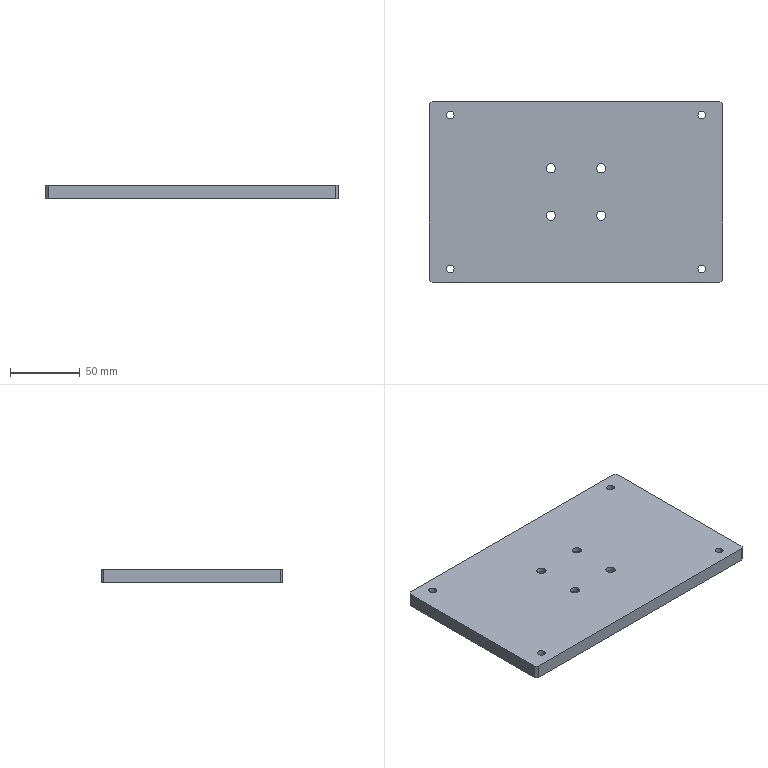Part | SolidWorks | features 3DProfileFeature 2, HoleWzd 2, Chamfer 1, Extrusion 1 | 1 solid | 50 faces | box 210 x 130 x 10 mm | volume 267698 mm3 | cylinder 32 | plane 18 | commonest cylinder face diameters 5.5 x8 6.6 x8 10 x8 11 x8
STEP:
#1=CARTESIAN_POINT('',(-85.,-55.,5.7));
#2=VERTEX_POINT('',#1);
#3=CARTESIAN_POINT('',(-95.,-55.,5.7));
#4=VERTEX_POINT('',#3);
#5=CARTESIAN_POINT('',(-90.,-55.,5.7));
#6=DIRECTION('',(0.,0.,-1.));
#7=DIRECTION('',(-1.,0.,0.));
#8=AXIS2_PLACEMENT_3D('',#5,#6,#7);
#9=CIRCLE('',#8,5.);
#10=EDGE_CURVE('',#2,#4,#9,.T.);
#11=ORIENTED_EDGE('',*,*,#10,.F.);
#12=CARTESIAN_POINT('',(-85.,-55.,0.));
#13=VERTEX_POINT('',#12);
#14=CARTESIAN_POINT('',(-85.,-55.,0.));
#15=DIRECTION('',(0.,0.,-1.));
#16=VECTOR('',#15,1000.);
#17=LINE('',#14,#16);
#18=EDGE_CURVE('',#2,#13,#17,.T.);
#19=ORIENTED_EDGE('',*,*,#18,.T.);
#20=CARTESIAN_POINT('',(-95.,-55.,0.));
#21=VERTEX_POINT('',#20);
#22=CARTESIAN_POINT('',(-90.,-55.,0.));
#23=DIRECTION('',(0.,0.,-1.));
#24=DIRECTION('',(-1.,0.,0.));
#25=AXIS2_PLACEMENT_3D('',#22,#23,#24);
#26=CIRCLE('',#25,5.);
#27=EDGE_CURVE('',#13,#21,#26,.T.);
#28=ORIENTED_EDGE('',*,*,#27,.T.);
#29=CARTESIAN_POINT('',(-95.,-55.,0.));
#30=DIRECTION('',(0.,0.,-1.));
#31=VECTOR('',#30,1000.);
#32=LINE('',#29,#31);
#33=EDGE_CURVE('',#4,#21,#32,.T.);
#34=ORIENTED_EDGE('',*,*,#33,.F.);
#35=EDGE_LOOP('',(#11,#19,#28,#34));
#36=FACE_OUTER_BOUND('',#35,.T.);
#37=CARTESIAN_POINT('',(-90.,-55.,0.));
#38=DIRECTION('',(0.,0.,-1.));
#39=DIRECTION('',(-1.,0.,0.));
#40=AXIS2_PLACEMENT_3D('',#37,#38,#39);
#41=CYLINDRICAL_SURFACE('',#40,5.);
#42=ADVANCED_FACE('',(#36),#41,.F.);
#43=CARTESIAN_POINT('',(-87.25,-55.,10.));
#44=VERTEX_POINT('',#43);
#45=CARTESIAN_POINT('',(-92.75,-55.,10.));
#46=VERTEX_POINT('',#45);
#47=CARTESIAN_POINT('',(-90.,-55.,10.));
#48=DIRECTION('',(0.,0.,-1.));
#49=DIRECTION('',(-1.,0.,0.));
#50=AXIS2_PLACEMENT_3D('',#47,#48,#49);
#51=CIRCLE('',#50,2.75);
#52=EDGE_CURVE('',#44,#46,#51,.T.);
#53=ORIENTED_EDGE('',*,*,#52,.F.);
#54=CARTESIAN_POINT('',(-87.25,-55.,5.7));
#55=VERTEX_POINT('',#54);
#56=CARTESIAN_POINT('',(-87.25,-55.,0.));
#57=DIRECTION('',(0.,0.,-1.));
#58=VECTOR('',#57,1000.);
#59=LINE('',#56,#58);
#60=EDGE_CURVE('',#44,#55,#59,.T.);
#61=ORIENTED_EDGE('',*,*,#60,.T.);
#62=CARTESIAN_POINT('',(-92.75,-55.,5.7));
#63=VERTEX_POINT('',#62);
#64=CARTESIAN_POINT('',(-90.,-55.,5.7));
#65=DIRECTION('',(0.,0.,-1.));
#66=DIRECTION('',(-1.,0.,0.));
#67=AXIS2_PLACEMENT_3D('',#64,#65,#66);
#68=CIRCLE('',#67,2.75);
#69=EDGE_CURVE('',#55,#63,#68,.T.);
#70=ORIENTED_EDGE('',*,*,#69,.T.);
#71=CARTESIAN_POINT('',(-92.75,-55.,0.));
#72=DIRECTION('',(0.,0.,-1.));
#73=VECTOR('',#72,1000.);
#74=LINE('',#71,#73);
#75=EDGE_CURVE('',#46,#63,#74,.T.);
#76=ORIENTED_EDGE('',*,*,#75,.F.);
#77=EDGE_LOOP('',(#53,#61,#70,#76));
#78=FACE_OUTER_BOUND('',#77,.T.);
#79=CARTESIAN_POINT('',(-90.,-55.,0.));
#80=DIRECTION('',(0.,0.,-1.));
#81=DIRECTION('',(-1.,0.,0.));
#82=AXIS2_PLACEMENT_3D('',#79,#80,#81);
#83=CYLINDRICAL_SURFACE('',#82,2.75);
#84=ADVANCED_FACE('',(#78),#83,.F.);
#85=CARTESIAN_POINT('',(-85.,55.,5.7));
#86=VERTEX_POINT('',#85);
#87=CARTESIAN_POINT('',(-95.,55.,5.7));
#88=VERTEX_POINT('',#87);
#89=CARTESIAN_POINT('',(-90.,55.,5.7));
#90=DIRECTION('',(0.,0.,-1.));
#91=DIRECTION('',(-1.,0.,0.));
#92=AXIS2_PLACEMENT_3D('',#89,#90,#91);
#93=CIRCLE('',#92,5.);
#94=EDGE_CURVE('',#86,#88,#93,.T.);
#95=ORIENTED_EDGE('',*,*,#94,.F.);
#96=CARTESIAN_POINT('',(-85.,55.,0.));
#97=VERTEX_POINT('',#96);
#98=CARTESIAN_POINT('',(-85.,55.,0.));
#99=DIRECTION('',(0.,0.,-1.));
#100=VECTOR('',#99,1000.);
#101=LINE('',#98,#100);
#102=EDGE_CURVE('',#86,#97,#101,.T.);
#103=ORIENTED_EDGE('',*,*,#102,.T.);
#104=CARTESIAN_POINT('',(-95.,55.,0.));
#105=VERTEX_POINT('',#104);
#106=CARTESIAN_POINT('',(-90.,55.,0.));
#107=DIRECTION('',(0.,0.,-1.));
#108=DIRECTION('',(-1.,0.,0.));
#109=AXIS2_PLACEMENT_3D('',#106,#107,#108);
#110=CIRCLE('',#109,5.);
#111=EDGE_CURVE('',#97,#105,#110,.T.);
#112=ORIENTED_EDGE('',*,*,#111,.T.);
#113=CARTESIAN_POINT('',(-95.,55.,0.));
#114=DIRECTION('',(0.,0.,-1.));
#115=VECTOR('',#114,1000.);
#116=LINE('',#113,#115);
#117=EDGE_CURVE('',#88,#105,#116,.T.);
#118=ORIENTED_EDGE('',*,*,#117,.F.);
#119=EDGE_LOOP('',(#95,#103,#112,#118));
#120=FACE_OUTER_BOUND('',#119,.T.);
#121=CARTESIAN_POINT('',(-90.,55.,0.));
#122=DIRECTION('',(0.,0.,-1.));
#123=DIRECTION('',(-1.,0.,0.));
#124=AXIS2_PLACEMENT_3D('',#121,#122,#123);
#125=CYLINDRICAL_SURFACE('',#124,5.);
#126=ADVANCED_FACE('',(#120),#125,.F.);
#127=CARTESIAN_POINT('',(-87.25,55.,10.));
#128=VERTEX_POINT('',#127);
#129=CARTESIAN_POINT('',(-92.75,55.,10.));
#130=VERTEX_POINT('',#129);
#131=CARTESIAN_POINT('',(-90.,55.,10.));
#132=DIRECTION('',(0.,0.,-1.));
#133=DIRECTION('',(-1.,0.,0.));
#134=AXIS2_PLACEMENT_3D('',#131,#132,#133);
#135=CIRCLE('',#134,2.75);
#136=EDGE_CURVE('',#128,#130,#135,.T.);
#137=ORIENTED_EDGE('',*,*,#136,.F.);
#138=CARTESIAN_POINT('',(-87.25,55.,5.7));
#139=VERTEX_POINT('',#138);
#140=CARTESIAN_POINT('',(-87.25,55.,0.));
#141=DIRECTION('',(0.,0.,-1.));
#142=VECTOR('',#141,1000.);
#143=LINE('',#140,#142);
#144=EDGE_CURVE('',#128,#139,#143,.T.);
#145=ORIENTED_EDGE('',*,*,#144,.T.);
#146=CARTESIAN_POINT('',(-92.75,55.,5.7));
#147=VERTEX_POINT('',#146);
#148=CARTESIAN_POINT('',(-90.,55.,5.7));
#149=DIRECTION('',(0.,0.,-1.));
#150=DIRECTION('',(-1.,0.,0.));
#151=AXIS2_PLACEMENT_3D('',#148,#149,#150);
#152=CIRCLE('',#151,2.75);
#153=EDGE_CURVE('',#139,#147,#152,.T.);
#154=ORIENTED_EDGE('',*,*,#153,.T.);
#155=CARTESIAN_POINT('',(-92.75,55.,0.));
#156=DIRECTION('',(0.,0.,-1.));
#157=VECTOR('',#156,1000.);
#158=LINE('',#155,#157);
#159=EDGE_CURVE('',#130,#147,#158,.T.);
#160=ORIENTED_EDGE('',*,*,#159,.F.);
#161=EDGE_LOOP('',(#137,#145,#154,#160));
#162=FACE_OUTER_BOUND('',#161,.T.);
#163=CARTESIAN_POINT('',(-90.,55.,0.));
#164=DIRECTION('',(0.,0.,-1.));
#165=DIRECTION('',(-1.,0.,0.));
#166=AXIS2_PLACEMENT_3D('',#163,#164,#165);
#167=CYLINDRICAL_SURFACE('',#166,2.75);
#168=ADVANCED_FACE('',(#162),#167,.F.);
#169=CARTESIAN_POINT('',(95.,55.,5.7));
#170=VERTEX_POINT('',#169);
#171=CARTESIAN_POINT('',(85.,55.,5.7));
#172=VERTEX_POINT('',#171);
#173=CARTESIAN_POINT('',(90.,55.,5.7));
#174=DIRECTION('',(0.,0.,-1.));
#175=DIRECTION('',(-1.,0.,0.));
#176=AXIS2_PLACEMENT_3D('',#173,#174,#175);
#177=CIRCLE('',#176,5.);
#178=EDGE_CURVE('',#170,#172,#177,.T.);
#179=ORIENTED_EDGE('',*,*,#178,.F.);
#180=CARTESIAN_POINT('',(95.,55.,0.));
#181=VERTEX_POINT('',#180);
#182=CARTESIAN_POINT('',(95.,55.,0.));
#183=DIRECTION('',(0.,0.,-1.));
#184=VECTOR('',#183,1000.);
#185=LINE('',#182,#184);
#186=EDGE_CURVE('',#170,#181,#185,.T.);
#187=ORIENTED_EDGE('',*,*,#186,.T.);
#188=CARTESIAN_POINT('',(85.,55.,0.));
#189=VERTEX_POINT('',#188);
#190=CARTESIAN_POINT('',(90.,55.,0.));
#191=DIRECTION('',(0.,0.,-1.));
#192=DIRECTION('',(-1.,0.,0.));
#193=AXIS2_PLACEMENT_3D('',#190,#191,#192);
#194=CIRCLE('',#193,5.);
#195=EDGE_CURVE('',#181,#189,#194,.T.);
#196=ORIENTED_EDGE('',*,*,#195,.T.);
#197=CARTESIAN_POINT('',(85.,55.,0.));
#198=DIRECTION('',(0.,0.,-1.));
#199=VECTOR('',#198,1000.);
#200=LINE('',#197,#199);
#201=EDGE_CURVE('',#172,#189,#200,.T.);
#202=ORIENTED_EDGE('',*,*,#201,.F.);
#203=EDGE_LOOP('',(#179,#187,#196,#202));
#204=FACE_OUTER_BOUND('',#203,.T.);
#205=CARTESIAN_POINT('',(90.,55.,0.));
#206=DIRECTION('',(0.,0.,-1.));
#207=DIRECTION('',(-1.,0.,0.));
#208=AXIS2_PLACEMENT_3D('',#205,#206,#207);
#209=CYLINDRICAL_SURFACE('',#208,5.);
#210=ADVANCED_FACE('',(#204),#209,.F.);
#211=CARTESIAN_POINT('',(92.75,55.,10.));
#212=VERTEX_POINT('',#211);
#213=CARTESIAN_POINT('',(87.25,55.,10.));
#214=VERTEX_POINT('',#213);
#215=CARTESIAN_POINT('',(90.,55.,10.));
#216=DIRECTION('',(0.,0.,-1.));
#217=DIRECTION('',(-1.,0.,0.));
#218=AXIS2_PLACEMENT_3D('',#215,#216,#217);
#219=CIRCLE('',#218,2.75);
#220=EDGE_CURVE('',#212,#214,#219,.T.);
#221=ORIENTED_EDGE('',*,*,#220,.F.);
#222=CARTESIAN_POINT('',(92.75,55.,5.7));
#223=VERTEX_POINT('',#222);
#224=CARTESIAN_POINT('',(92.75,55.,0.));
#225=DIRECTION('',(0.,0.,-1.));
#226=VECTOR('',#225,1000.);
#227=LINE('',#224,#226);
#228=EDGE_CURVE('',#212,#223,#227,.T.);
#229=ORIENTED_EDGE('',*,*,#228,.T.);
#230=CARTESIAN_POINT('',(87.25,55.,5.7));
#231=VERTEX_POINT('',#230);
#232=CARTESIAN_POINT('',(90.,55.,5.7));
#233=DIRECTION('',(0.,0.,-1.));
#234=DIRECTION('',(-1.,0.,0.));
#235=AXIS2_PLACEMENT_3D('',#232,#233,#234);
#236=CIRCLE('',#235,2.75);
#237=EDGE_CURVE('',#223,#231,#236,.T.);
#238=ORIENTED_EDGE('',*,*,#237,.T.);
#239=CARTESIAN_POINT('',(87.25,55.,0.));
#240=DIRECTION('',(0.,0.,-1.));
#241=VECTOR('',#240,1000.);
#242=LINE('',#239,#241);
#243=EDGE_CURVE('',#214,#231,#242,.T.);
#244=ORIENTED_EDGE('',*,*,#243,.F.);
#245=EDGE_LOOP('',(#221,#229,#238,#244));
#246=FACE_OUTER_BOUND('',#245,.T.);
#247=CARTESIAN_POINT('',(90.,55.,0.));
#248=DIRECTION('',(0.,0.,-1.));
#249=DIRECTION('',(-1.,0.,0.));
#250=AXIS2_PLACEMENT_3D('',#247,#248,#249);
#251=CYLINDRICAL_SURFACE('',#250,2.75);
#252=ADVANCED_FACE('',(#246),#251,.F.);
#253=CARTESIAN_POINT('',(95.,-55.,5.7));
#254=VERTEX_POINT('',#253);
#255=CARTESIAN_POINT('',(85.,-55.,5.7));
#256=VERTEX_POINT('',#255);
#257=CARTESIAN_POINT('',(90.,-55.,5.7));
#258=DIRECTION('',(0.,0.,-1.));
#259=DIRECTION('',(-1.,0.,0.));
#260=AXIS2_PLACEMENT_3D('',#257,#258,#259);
#261=CIRCLE('',#260,5.);
#262=EDGE_CURVE('',#254,#256,#261,.T.);
#263=ORIENTED_EDGE('',*,*,#262,.F.);
#264=CARTESIAN_POINT('',(95.,-55.,0.));
#265=VERTEX_POINT('',#264);
#266=CARTESIAN_POINT('',(95.,-55.,0.));
#267=DIRECTION('',(0.,0.,-1.));
#268=VECTOR('',#267,1000.);
#269=LINE('',#266,#268);
#270=EDGE_CURVE('',#254,#265,#269,.T.);
#271=ORIENTED_EDGE('',*,*,#270,.T.);
#272=CARTESIAN_POINT('',(85.,-55.,0.));
#273=VERTEX_POINT('',#272);
#274=CARTESIAN_POINT('',(90.,-55.,0.));
#275=DIRECTION('',(0.,0.,-1.));
#276=DIRECTION('',(-1.,0.,0.));
#277=AXIS2_PLACEMENT_3D('',#274,#275,#276);
#278=CIRCLE('',#277,5.);
#279=EDGE_CURVE('',#265,#273,#278,.T.);
#280=ORIENTED_EDGE('',*,*,#279,.T.);
#281=CARTESIAN_POINT('',(85.,-55.,0.));
#282=DIRECTION('',(0.,0.,-1.));
#283=VECTOR('',#282,1000.);
#284=LINE('',#281,#283);
#285=EDGE_CURVE('',#256,#273,#284,.T.);
#286=ORIENTED_EDGE('',*,*,#285,.F.);
#287=EDGE_LOOP('',(#263,#271,#280,#286));
#288=FACE_OUTER_BOUND('',#287,.T.);
#289=CARTESIAN_POINT('',(90.,-55.,0.));
#290=DIRECTION('',(0.,0.,-1.));
#291=DIRECTION('',(-1.,0.,0.));
#292=AXIS2_PLACEMENT_3D('',#289,#290,#291);
#293=CYLINDRICAL_SURFACE('',#292,5.);
#294=ADVANCED_FACE('',(#288),#293,.F.);
#295=CARTESIAN_POINT('',(92.75,-55.,10.));
#296=VERTEX_POINT('',#295);
#297=CARTESIAN_POINT('',(87.25,-55.,10.));
#298=VERTEX_POINT('',#297);
#299=CARTESIAN_POINT('',(90.,-55.,10.));
#300=DIRECTION('',(0.,0.,-1.));
#301=DIRECTION('',(-1.,0.,0.));
#302=AXIS2_PLACEMENT_3D('',#299,#300,#301);
#303=CIRCLE('',#302,2.75);
#304=EDGE_CURVE('',#296,#298,#303,.T.);
#305=ORIENTED_EDGE('',*,*,#304,.F.);
#306=CARTESIAN_POINT('',(92.75,-55.,5.7));
#307=VERTEX_POINT('',#306);
#308=CARTESIAN_POINT('',(92.75,-55.,0.));
#309=DIRECTION('',(0.,0.,-1.));
#310=VECTOR('',#309,1000.);
#311=LINE('',#308,#310);
#312=EDGE_CURVE('',#296,#307,#311,.T.);
#313=ORIENTED_EDGE('',*,*,#312,.T.);
#314=CARTESIAN_POINT('',(87.25,-55.,5.7));
#315=VERTEX_POINT('',#314);
#316=CARTESIAN_POINT('',(90.,-55.,5.7));
#317=DIRECTION('',(0.,0.,-1.));
#318=DIRECTION('',(-1.,0.,0.));
#319=AXIS2_PLACEMENT_3D('',#316,#317,#318);
#320=CIRCLE('',#319,2.75);
#321=EDGE_CURVE('',#307,#315,#320,.T.);
#322=ORIENTED_EDGE('',*,*,#321,.T.);
#323=CARTESIAN_POINT('',(87.25,-55.,0.));
#324=DIRECTION('',(0.,0.,-1.));
#325=VECTOR('',#324,1000.);
#326=LINE('',#323,#325);
#327=EDGE_CURVE('',#298,#315,#326,.T.);
#328=ORIENTED_EDGE('',*,*,#327,.F.);
#329=EDGE_LOOP('',(#305,#313,#322,#328));
#330=FACE_OUTER_BOUND('',#329,.T.);
#331=CARTESIAN_POINT('',(90.,-55.,0.));
#332=DIRECTION('',(0.,0.,-1.));
#333=DIRECTION('',(-1.,0.,0.));
#334=AXIS2_PLACEMENT_3D('',#331,#332,#333);
#335=CYLINDRICAL_SURFACE('',#334,2.75);
#336=ADVANCED_FACE('',(#330),#335,.F.);
#337=CARTESIAN_POINT('',(-12.5,-17.,6.8));
#338=VERTEX_POINT('',#337);
#339=CARTESIAN_POINT('',(-23.5,-17.,6.8));
#340=VERTEX_POINT('',#339);
#341=CARTESIAN_POINT('',(-18.,-17.,6.8));
#342=DIRECTION('',(0.,0.,-1.));
#343=DIRECTION('',(-1.,0.,0.));
#344=AXIS2_PLACEMENT_3D('',#341,#342,#343);
#345=CIRCLE('',#344,5.5);
#346=EDGE_CURVE('',#338,#340,#345,.T.);
#347=ORIENTED_EDGE('',*,*,#346,.F.);
#348=CARTESIAN_POINT('',(-12.5,-17.,0.));
#349=VERTEX_POINT('',#348);
#350=CARTESIAN_POINT('',(-12.5,-17.,0.));
#351=DIRECTION('',(0.,0.,-1.));
#352=VECTOR('',#351,1000.);
#353=LINE('',#350,#352);
#354=EDGE_CURVE('',#338,#349,#353,.T.);
#355=ORIENTED_EDGE('',*,*,#354,.T.);
#356=CARTESIAN_POINT('',(-23.5,-17.,0.));
#357=VERTEX_POINT('',#356);
#358=CARTESIAN_POINT('',(-18.,-17.,0.));
#359=DIRECTION('',(0.,0.,-1.));
#360=DIRECTION('',(-1.,0.,0.));
#361=AXIS2_PLACEMENT_3D('',#358,#359,#360);
#362=CIRCLE('',#361,5.5);
#363=EDGE_CURVE('',#349,#357,#362,.T.);
#364=ORIENTED_EDGE('',*,*,#363,.T.);
#365=CARTESIAN_POINT('',(-23.5,-17.,0.));
#366=DIRECTION('',(0.,0.,-1.));
#367=VECTOR('',#366,1000.);
#368=LINE('',#365,#367);
#369=EDGE_CURVE('',#340,#357,#368,.T.);
#370=ORIENTED_EDGE('',*,*,#369,.F.);
#371=EDGE_LOOP('',(#347,#355,#364,#370));
#372=FACE_OUTER_BOUND('',#371,.T.);
#373=CARTESIAN_POINT('',(-18.,-17.,0.));
#374=DIRECTION('',(0.,0.,-1.));
#375=DIRECTION('',(-1.,0.,0.));
#376=AXIS2_PLACEMENT_3D('',#373,#374,#375);
#377=CYLINDRICAL_SURFACE('',#376,5.5);
#378=ADVANCED_FACE('',(#372),#377,.F.);
#379=CARTESIAN_POINT('',(-14.7,-17.,10.));
#380=VERTEX_POINT('',#379);
#381=CARTESIAN_POINT('',(-21.3,-17.,10.));
#382=VERTEX_POINT('',#381);
#383=CARTESIAN_POINT('',(-18.,-17.,10.));
#384=DIRECTION('',(0.,0.,-1.));
#385=DIRECTION('',(-1.,0.,0.));
#386=AXIS2_PLACEMENT_3D('',#383,#384,#385);
#387=CIRCLE('',#386,3.3);
#388=EDGE_CURVE('',#380,#382,#387,.T.);
#389=ORIENTED_EDGE('',*,*,#388,.F.);
#390=CARTESIAN_POINT('',(-14.7,-17.,6.8));
#391=VERTEX_POINT('',#390);
#392=CARTESIAN_POINT('',(-14.7,-17.,0.));
#393=DIRECTION('',(0.,0.,-1.));
#394=VECTOR('',#393,1000.);
#395=LINE('',#392,#394);
#396=EDGE_CURVE('',#380,#391,#395,.T.);
#397=ORIENTED_EDGE('',*,*,#396,.T.);
#398=CARTESIAN_POINT('',(-21.3,-17.,6.8));
#399=VERTEX_POINT('',#398);
#400=CARTESIAN_POINT('',(-18.,-17.,6.8));
#401=DIRECTION('',(0.,0.,-1.));
#402=DIRECTION('',(-1.,0.,0.));
#403=AXIS2_PLACEMENT_3D('',#400,#401,#402);
#404=CIRCLE('',#403,3.3);
#405=EDGE_CURVE('',#391,#399,#404,.T.);
#406=ORIENTED_EDGE('',*,*,#405,.T.);
#407=CARTESIAN_POINT('',(-21.3,-17.,0.));
#408=DIRECTION('',(0.,0.,-1.));
#409=VECTOR('',#408,1000.);
#410=LINE('',#407,#409);
#411=EDGE_CURVE('',#382,#399,#410,.T.);
#412=ORIENTED_EDGE('',*,*,#411,.F.);
#413=EDGE_LOOP('',(#389,#397,#406,#412));
#414=FACE_OUTER_BOUND('',#413,.T.);
#415=CARTESIAN_POINT('',(-18.,-17.,0.));
#416=DIRECTION('',(0.,0.,-1.));
#417=DIRECTION('',(-1.,0.,0.));
#418=AXIS2_PLACEMENT_3D('',#415,#416,#417);
#419=CYLINDRICAL_SURFACE('',#418,3.3);
#420=ADVANCED_FACE('',(#414),#419,.F.);
#421=CARTESIAN_POINT('',(23.5,-17.,6.8));
#422=VERTEX_POINT('',#421);
#423=CARTESIAN_POINT('',(12.5,-17.,6.8));
#424=VERTEX_POINT('',#423);
#425=CARTESIAN_POINT('',(18.,-17.,6.8));
#426=DIRECTION('',(0.,0.,-1.));
#427=DIRECTION('',(-1.,0.,0.));
#428=AXIS2_PLACEMENT_3D('',#425,#426,#427);
#429=CIRCLE('',#428,5.5);
#430=EDGE_CURVE('',#422,#424,#429,.T.);
#431=ORIENTED_EDGE('',*,*,#430,.F.);
#432=CARTESIAN_POINT('',(23.5,-17.,0.));
#433=VERTEX_POINT('',#432);
#434=CARTESIAN_POINT('',(23.5,-17.,0.));
#435=DIRECTION('',(0.,0.,-1.));
#436=VECTOR('',#435,1000.);
#437=LINE('',#434,#436);
#438=EDGE_CURVE('',#422,#433,#437,.T.);
#439=ORIENTED_EDGE('',*,*,#438,.T.);
#440=CARTESIAN_POINT('',(12.5,-17.,0.));
#441=VERTEX_POINT('',#440);
#442=CARTESIAN_POINT('',(18.,-17.,0.));
#443=DIRECTION('',(0.,0.,-1.));
#444=DIRECTION('',(-1.,0.,0.));
#445=AXIS2_PLACEMENT_3D('',#442,#443,#444);
#446=CIRCLE('',#445,5.5);
#447=EDGE_CURVE('',#433,#441,#446,.T.);
#448=ORIENTED_EDGE('',*,*,#447,.T.);
#449=CARTESIAN_POINT('',(12.5,-17.,0.));
#450=DIRECTION('',(0.,0.,-1.));
#451=VECTOR('',#450,1000.);
#452=LINE('',#449,#451);
#453=EDGE_CURVE('',#424,#441,#452,.T.);
#454=ORIENTED_EDGE('',*,*,#453,.F.);
#455=EDGE_LOOP('',(#431,#439,#448,#454));
#456=FACE_OUTER_BOUND('',#455,.T.);
#457=CARTESIAN_POINT('',(18.,-17.,0.));
#458=DIRECTION('',(0.,0.,-1.));
#459=DIRECTION('',(-1.,0.,0.));
#460=AXIS2_PLACEMENT_3D('',#457,#458,#459);
#461=CYLINDRICAL_SURFACE('',#460,5.5);
#462=ADVANCED_FACE('',(#456),#461,.F.);
#463=CARTESIAN_POINT('',(21.3,-17.,10.));
#464=VERTEX_POINT('',#463);
#465=CARTESIAN_POINT('',(14.7,-17.,10.));
#466=VERTEX_POINT('',#465);
#467=CARTESIAN_POINT('',(18.,-17.,10.));
#468=DIRECTION('',(0.,0.,-1.));
#469=DIRECTION('',(-1.,0.,0.));
#470=AXIS2_PLACEMENT_3D('',#467,#468,#469);
#471=CIRCLE('',#470,3.3);
#472=EDGE_CURVE('',#464,#466,#471,.T.);
#473=ORIENTED_EDGE('',*,*,#472,.F.);
#474=CARTESIAN_POINT('',(21.3,-17.,6.8));
#475=VERTEX_POINT('',#474);
#476=CARTESIAN_POINT('',(21.3,-17.,0.));
#477=DIRECTION('',(0.,0.,-1.));
#478=VECTOR('',#477,1000.);
#479=LINE('',#476,#478);
#480=EDGE_CURVE('',#464,#475,#479,.T.);
#481=ORIENTED_EDGE('',*,*,#480,.T.);
#482=CARTESIAN_POINT('',(14.7,-17.,6.8));
#483=VERTEX_POINT('',#482);
#484=CARTESIAN_POINT('',(18.,-17.,6.8));
#485=DIRECTION('',(0.,0.,-1.));
#486=DIRECTION('',(-1.,0.,0.));
#487=AXIS2_PLACEMENT_3D('',#484,#485,#486);
#488=CIRCLE('',#487,3.3);
#489=EDGE_CURVE('',#475,#483,#488,.T.);
#490=ORIENTED_EDGE('',*,*,#489,.T.);
#491=CARTESIAN_POINT('',(14.7,-17.,0.));
#492=DIRECTION('',(0.,0.,-1.));
#493=VECTOR('',#492,1000.);
#494=LINE('',#491,#493);
#495=EDGE_CURVE('',#466,#483,#494,.T.);
#496=ORIENTED_EDGE('',*,*,#495,.F.);
#497=EDGE_LOOP('',(#473,#481,#490,#496));
#498=FACE_OUTER_BOUND('',#497,.T.);
#499=CARTESIAN_POINT('',(18.,-17.,0.));
#500=DIRECTION('',(0.,0.,-1.));
#501=DIRECTION('',(-1.,0.,0.));
#502=AXIS2_PLACEMENT_3D('',#499,#500,#501);
#503=CYLINDRICAL_SURFACE('',#502,3.3);
#504=ADVANCED_FACE('',(#498),#503,.F.);
#505=CARTESIAN_POINT('',(23.5,17.,6.8));
#506=VERTEX_POINT('',#505);
#507=CARTESIAN_POINT('',(12.5,17.,6.8));
#508=VERTEX_POINT('',#507);
#509=CARTESIAN_POINT('',(18.,17.,6.8));
#510=DIRECTION('',(0.,0.,-1.));
#511=DIRECTION('',(-1.,0.,0.));
#512=AXIS2_PLACEMENT_3D('',#509,#510,#511);
#513=CIRCLE('',#512,5.5);
#514=EDGE_CURVE('',#506,#508,#513,.T.);
#515=ORIENTED_EDGE('',*,*,#514,.F.);
#516=CARTESIAN_POINT('',(23.5,17.,0.));
#517=VERTEX_POINT('',#516);
#518=CARTESIAN_POINT('',(23.5,17.,0.));
#519=DIRECTION('',(0.,0.,-1.));
#520=VECTOR('',#519,1000.);
#521=LINE('',#518,#520);
#522=EDGE_CURVE('',#506,#517,#521,.T.);
#523=ORIENTED_EDGE('',*,*,#522,.T.);
#524=CARTESIAN_POINT('',(12.5,17.,0.));
#525=VERTEX_POINT('',#524);
#526=CARTESIAN_POINT('',(18.,17.,0.));
#527=DIRECTION('',(0.,0.,-1.));
#528=DIRECTION('',(-1.,0.,0.));
#529=AXIS2_PLACEMENT_3D('',#526,#527,#528);
#530=CIRCLE('',#529,5.5);
#531=EDGE_CURVE('',#517,#525,#530,.T.);
#532=ORIENTED_EDGE('',*,*,#531,.T.);
#533=CARTESIAN_POINT('',(12.5,17.,0.));
#534=DIRECTION('',(0.,0.,-1.));
#535=VECTOR('',#534,1000.);
#536=LINE('',#533,#535);
#537=EDGE_CURVE('',#508,#525,#536,.T.);
#538=ORIENTED_EDGE('',*,*,#537,.F.);
#539=EDGE_LOOP('',(#515,#523,#532,#538));
#540=FACE_OUTER_BOUND('',#539,.T.);
#541=CARTESIAN_POINT('',(18.,17.,0.));
#542=DIRECTION('',(0.,0.,-1.));
#543=DIRECTION('',(-1.,0.,0.));
#544=AXIS2_PLACEMENT_3D('',#541,#542,#543);
#545=CYLINDRICAL_SURFACE('',#544,5.5);
#546=ADVANCED_FACE('',(#540),#545,.F.);
#547=CARTESIAN_POINT('',(21.3,17.,10.));
#548=VERTEX_POINT('',#547);
#549=CARTESIAN_POINT('',(14.7,17.,10.));
#550=VERTEX_POINT('',#549);
#551=CARTESIAN_POINT('',(18.,17.,10.));
#552=DIRECTION('',(0.,0.,-1.));
#553=DIRECTION('',(-1.,0.,0.));
#554=AXIS2_PLACEMENT_3D('',#551,#552,#553);
#555=CIRCLE('',#554,3.3);
#556=EDGE_CURVE('',#548,#550,#555,.T.);
#557=ORIENTED_EDGE('',*,*,#556,.F.);
#558=CARTESIAN_POINT('',(21.3,17.,6.8));
#559=VERTEX_POINT('',#558);
#560=CARTESIAN_POINT('',(21.3,17.,0.));
#561=DIRECTION('',(0.,0.,-1.));
#562=VECTOR('',#561,1000.);
#563=LINE('',#560,#562);
#564=EDGE_CURVE('',#548,#559,#563,.T.);
#565=ORIENTED_EDGE('',*,*,#564,.T.);
#566=CARTESIAN_POINT('',(14.7,17.,6.8));
#567=VERTEX_POINT('',#566);
#568=CARTESIAN_POINT('',(18.,17.,6.8));
#569=DIRECTION('',(0.,0.,-1.));
#570=DIRECTION('',(-1.,0.,0.));
#571=AXIS2_PLACEMENT_3D('',#568,#569,#570);
#572=CIRCLE('',#571,3.3);
#573=EDGE_CURVE('',#559,#567,#572,.T.);
#574=ORIENTED_EDGE('',*,*,#573,.T.);
#575=CARTESIAN_POINT('',(14.7,17.,0.));
#576=DIRECTION('',(0.,0.,-1.));
#577=VECTOR('',#576,1000.);
#578=LINE('',#575,#577);
#579=EDGE_CURVE('',#550,#567,#578,.T.);
#580=ORIENTED_EDGE('',*,*,#579,.F.);
#581=EDGE_LOOP('',(#557,#565,#574,#580));
#582=FACE_OUTER_BOUND('',#581,.T.);
#583=CARTESIAN_POINT('',(18.,17.,0.));
#584=DIRECTION('',(0.,0.,-1.));
#585=DIRECTION('',(-1.,0.,0.));
#586=AXIS2_PLACEMENT_3D('',#583,#584,#585);
#587=CYLINDRICAL_SURFACE('',#586,3.3);
#588=ADVANCED_FACE('',(#582),#587,.F.);
#589=CARTESIAN_POINT('',(-12.5,17.,6.8));
#590=VERTEX_POINT('',#589);
#591=CARTESIAN_POINT('',(-23.5,17.,6.8));
#592=VERTEX_POINT('',#591);
#593=CARTESIAN_POINT('',(-18.,17.,6.8));
#594=DIRECTION('',(0.,0.,-1.));
#595=DIRECTION('',(-1.,0.,0.));
#596=AXIS2_PLACEMENT_3D('',#593,#594,#595);
#597=CIRCLE('',#596,5.5);
#598=EDGE_CURVE('',#590,#592,#597,.T.);
#599=ORIENTED_EDGE('',*,*,#598,.F.);
#600=CARTESIAN_POINT('',(-12.5,17.,0.));
#601=VERTEX_POINT('',#600);
#602=CARTESIAN_POINT('',(-12.5,17.,0.));
#603=DIRECTION('',(0.,0.,-1.));
#604=VECTOR('',#603,1000.);
#605=LINE('',#602,#604);
#606=EDGE_CURVE('',#590,#601,#605,.T.);
#607=ORIENTED_EDGE('',*,*,#606,.T.);
#608=CARTESIAN_POINT('',(-23.5,17.,0.));
#609=VERTEX_POINT('',#608);
#610=CARTESIAN_POINT('',(-18.,17.,0.));
#611=DIRECTION('',(0.,0.,-1.));
#612=DIRECTION('',(-1.,0.,0.));
#613=AXIS2_PLACEMENT_3D('',#610,#611,#612);
#614=CIRCLE('',#613,5.5);
#615=EDGE_CURVE('',#601,#609,#614,.T.);
#616=ORIENTED_EDGE('',*,*,#615,.T.);
#617=CARTESIAN_POINT('',(-23.5,17.,0.));
#618=DIRECTION('',(0.,0.,-1.));
#619=VECTOR('',#618,1000.);
#620=LINE('',#617,#619);
#621=EDGE_CURVE('',#592,#609,#620,.T.);
#622=ORIENTED_EDGE('',*,*,#621,.F.);
#623=EDGE_LOOP('',(#599,#607,#616,#622));
#624=FACE_OUTER_BOUND('',#623,.T.);
#625=CARTESIAN_POINT('',(-18.,17.,0.));
#626=DIRECTION('',(0.,0.,-1.));
#627=DIRECTION('',(-1.,0.,0.));
#628=AXIS2_PLACEMENT_3D('',#625,#626,#627);
#629=CYLINDRICAL_SURFACE('',#628,5.5);
#630=ADVANCED_FACE('',(#624),#629,.F.);
#631=CARTESIAN_POINT('',(-14.7,17.,10.));
#632=VERTEX_POINT('',#631);
#633=CARTESIAN_POINT('',(-21.3,17.,10.));
#634=VERTEX_POINT('',#633);
#635=CARTESIAN_POINT('',(-18.,17.,10.));
#636=DIRECTION('',(0.,0.,-1.));
#637=DIRECTION('',(-1.,0.,0.));
#638=AXIS2_PLACEMENT_3D('',#635,#636,#637);
#639=CIRCLE('',#638,3.3);
#640=EDGE_CURVE('',#632,#634,#639,.T.);
#641=ORIENTED_EDGE('',*,*,#640,.F.);
#642=CARTESIAN_POINT('',(-14.7,17.,6.8));
#643=VERTEX_POINT('',#642);
#644=CARTESIAN_POINT('',(-14.7,17.,0.));
#645=DIRECTION('',(0.,0.,-1.));
#646=VECTOR('',#645,1000.);
#647=LINE('',#644,#646);
#648=EDGE_CURVE('',#632,#643,#647,.T.);
#649=ORIENTED_EDGE('',*,*,#648,.T.);
#650=CARTESIAN_POINT('',(-21.3,17.,6.8));
#651=VERTEX_POINT('',#650);
#652=CARTESIAN_POINT('',(-18.,17.,6.8));
#653=DIRECTION('',(0.,0.,-1.));
#654=DIRECTION('',(-1.,0.,0.));
#655=AXIS2_PLACEMENT_3D('',#652,#653,#654);
#656=CIRCLE('',#655,3.3);
#657=EDGE_CURVE('',#643,#651,#656,.T.);
#658=ORIENTED_EDGE('',*,*,#657,.T.);
#659=CARTESIAN_POINT('',(-21.3,17.,0.));
#660=DIRECTION('',(0.,0.,-1.));
#661=VECTOR('',#660,1000.);
#662=LINE('',#659,#661);
#663=EDGE_CURVE('',#634,#651,#662,.T.);
#664=ORIENTED_EDGE('',*,*,#663,.F.);
#665=EDGE_LOOP('',(#641,#649,#658,#664));
#666=FACE_OUTER_BOUND('',#665,.T.);
#667=CARTESIAN_POINT('',(-18.,17.,0.));
#668=DIRECTION('',(0.,0.,-1.));
#669=DIRECTION('',(-1.,0.,0.));
#670=AXIS2_PLACEMENT_3D('',#667,#668,#669);
#671=CYLINDRICAL_SURFACE('',#670,3.3);
#672=ADVANCED_FACE('',(#666),#671,.F.);
#673=CARTESIAN_POINT('',(105.,-63.,10.));
#674=VERTEX_POINT('',#673);
#675=CARTESIAN_POINT('',(105.,63.,10.));
#676=VERTEX_POINT('',#675);
#677=CARTESIAN_POINT('',(105.,-65.,10.));
#678=DIRECTION('',(0.,1.,0.));
#679=VECTOR('',#678,1000.);
#680=LINE('',#677,#679);
#681=EDGE_CURVE('',#674,#676,#680,.T.);
#682=ORIENTED_EDGE('',*,*,#681,.F.);
#683=CARTESIAN_POINT('',(105.,-63.,0.));
#684=VERTEX_POINT('',#683);
#685=CARTESIAN_POINT('',(105.,-63.,10.));
#686=DIRECTION('',(0.,0.,-1.));
#687=VECTOR('',#686,1000.);
#688=LINE('',#685,#687);
#689=EDGE_CURVE('',#674,#684,#688,.T.);
#690=ORIENTED_EDGE('',*,*,#689,.T.);
#691=CARTESIAN_POINT('',(105.,63.,0.));
#692=VERTEX_POINT('',#691);
#693=CARTESIAN_POINT('',(105.,-65.,0.));
#694=DIRECTION('',(0.,1.,0.));
#695=VECTOR('',#694,1000.);
#696=LINE('',#693,#695);
#697=EDGE_CURVE('',#684,#692,#696,.T.);
#698=ORIENTED_EDGE('',*,*,#697,.T.);
#699=CARTESIAN_POINT('',(105.,63.,10.));
#700=DIRECTION('',(0.,0.,1.));
#701=VECTOR('',#700,1000.);
#702=LINE('',#699,#701);
#703=EDGE_CURVE('',#692,#676,#702,.T.);
#704=ORIENTED_EDGE('',*,*,#703,.T.);
#705=EDGE_LOOP('',(#682,#690,#698,#704));
#706=FACE_OUTER_BOUND('',#705,.T.);
#707=CARTESIAN_POINT('',(105.,-65.,10.));
#708=DIRECTION('',(-1.,0.,0.));
#709=DIRECTION('',(0.,0.,1.));
#710=AXIS2_PLACEMENT_3D('',#707,#708,#709);
#711=PLANE('',#710);
#712=ADVANCED_FACE('',(#706),#711,.F.);
#713=CARTESIAN_POINT('',(103.,65.,0.));
#714=VERTEX_POINT('',#713);
#715=CARTESIAN_POINT('',(-103.,65.,0.));
#716=VERTEX_POINT('',#715);
#717=CARTESIAN_POINT('',(-105.,65.,0.));
#718=DIRECTION('',(-1.,0.,0.));
#719=VECTOR('',#718,1000.);
#720=LINE('',#717,#719);
#721=EDGE_CURVE('',#714,#716,#720,.T.);
#722=ORIENTED_EDGE('',*,*,#721,.T.);
#723=CARTESIAN_POINT('',(-103.,65.,10.));
#724=VERTEX_POINT('',#723);
#725=CARTESIAN_POINT('',(-103.,65.,10.));
#726=DIRECTION('',(0.,0.,1.));
#727=VECTOR('',#726,1000.);
#728=LINE('',#725,#727);
#729=EDGE_CURVE('',#716,#724,#728,.T.);
#730=ORIENTED_EDGE('',*,*,#729,.T.);
#731=CARTESIAN_POINT('',(103.,65.,10.));
#732=VERTEX_POINT('',#731);
#733=CARTESIAN_POINT('',(-105.,65.,10.));
#734=DIRECTION('',(-1.,0.,0.));
#735=VECTOR('',#734,1000.);
#736=LINE('',#733,#735);
#737=EDGE_CURVE('',#732,#724,#736,.T.);
#738=ORIENTED_EDGE('',*,*,#737,.F.);
#739=CARTESIAN_POINT('',(103.,65.,10.));
#740=DIRECTION('',(0.,0.,-1.));
#741=VECTOR('',#740,1000.);
#742=LINE('',#739,#741);
#743=EDGE_CURVE('',#732,#714,#742,.T.);
#744=ORIENTED_EDGE('',*,*,#743,.T.);
#745=EDGE_LOOP('',(#722,#730,#738,#744));
#746=FACE_OUTER_BOUND('',#745,.T.);
#747=CARTESIAN_POINT('',(-105.,65.,10.));
#748=DIRECTION('',(0.,-1.,0.));
#749=DIRECTION('',(0.,0.,-1.));
#750=AXIS2_PLACEMENT_3D('',#747,#748,#749);
#751=PLANE('',#750);
#752=ADVANCED_FACE('',(#746),#751,.F.);
#753=CARTESIAN_POINT('',(-105.,63.,0.));
#754=VERTEX_POINT('',#753);
#755=CARTESIAN_POINT('',(-105.,-63.,0.));
#756=VERTEX_POINT('',#755);
#757=CARTESIAN_POINT('',(-105.,-65.,0.));
#758=DIRECTION('',(0.,-1.,0.));
#759=VECTOR('',#758,1000.);
#760=LINE('',#757,#759);
#761=EDGE_CURVE('',#754,#756,#760,.T.);
#762=ORIENTED_EDGE('',*,*,#761,.T.);
#763=CARTESIAN_POINT('',(-105.,-63.,10.));
#764=VERTEX_POINT('',#763);
#765=CARTESIAN_POINT('',(-105.,-63.,10.));
#766=DIRECTION('',(0.,0.,1.));
#767=VECTOR('',#766,1000.);
#768=LINE('',#765,#767);
#769=EDGE_CURVE('',#756,#764,#768,.T.);
#770=ORIENTED_EDGE('',*,*,#769,.T.);
#771=CARTESIAN_POINT('',(-105.,63.,10.));
#772=VERTEX_POINT('',#771);
#773=CARTESIAN_POINT('',(-105.,-65.,10.));
#774=DIRECTION('',(0.,-1.,0.));
#775=VECTOR('',#774,1000.);
#776=LINE('',#773,#775);
#777=EDGE_CURVE('',#772,#764,#776,.T.);
#778=ORIENTED_EDGE('',*,*,#777,.F.);
#779=CARTESIAN_POINT('',(-105.,63.,10.));
#780=DIRECTION('',(0.,0.,-1.));
#781=VECTOR('',#780,1000.);
#782=LINE('',#779,#781);
#783=EDGE_CURVE('',#772,#754,#782,.T.);
#784=ORIENTED_EDGE('',*,*,#783,.T.);
#785=EDGE_LOOP('',(#762,#770,#778,#784));
#786=FACE_OUTER_BOUND('',#785,.T.);
#787=CARTESIAN_POINT('',(-105.,-65.,10.));
#788=DIRECTION('',(1.,0.,0.));
#789=DIRECTION('',(0.,0.,-1.));
#790=AXIS2_PLACEMENT_3D('',#787,#788,#789);
#791=PLANE('',#790);
#792=ADVANCED_FACE('',(#786),#791,.F.);
#793=CARTESIAN_POINT('',(-103.,-65.,10.));
#794=VERTEX_POINT('',#793);
#795=CARTESIAN_POINT('',(103.,-65.,10.));
#796=VERTEX_POINT('',#795);
#797=CARTESIAN_POINT('',(-105.,-65.,10.));
#798=DIRECTION('',(1.,0.,0.));
#799=VECTOR('',#798,1000.);
#800=LINE('',#797,#799);
#801=EDGE_CURVE('',#794,#796,#800,.T.);
#802=ORIENTED_EDGE('',*,*,#801,.F.);
#803=CARTESIAN_POINT('',(-103.,-65.,0.));
#804=VERTEX_POINT('',#803);
#805=CARTESIAN_POINT('',(-103.,-65.,10.));
#806=DIRECTION('',(0.,0.,-1.));
#807=VECTOR('',#806,1000.);
#808=LINE('',#805,#807);
#809=EDGE_CURVE('',#794,#804,#808,.T.);
#810=ORIENTED_EDGE('',*,*,#809,.T.);
#811=CARTESIAN_POINT('',(103.,-65.,0.));
#812=VERTEX_POINT('',#811);
#813=CARTESIAN_POINT('',(-105.,-65.,0.));
#814=DIRECTION('',(1.,0.,0.));
#815=VECTOR('',#814,1000.);
#816=LINE('',#813,#815);
#817=EDGE_CURVE('',#804,#812,#816,.T.);
#818=ORIENTED_EDGE('',*,*,#817,.T.);
#819=CARTESIAN_POINT('',(103.,-65.,10.));
#820=DIRECTION('',(0.,0.,1.));
#821=VECTOR('',#820,1000.);
#822=LINE('',#819,#821);
#823=EDGE_CURVE('',#812,#796,#822,.T.);
#824=ORIENTED_EDGE('',*,*,#823,.T.);
#825=EDGE_LOOP('',(#802,#810,#818,#824));
#826=FACE_OUTER_BOUND('',#825,.T.);
#827=CARTESIAN_POINT('',(-105.,-65.,10.));
#828=DIRECTION('',(0.,1.,0.));
#829=DIRECTION('',(0.,0.,1.));
#830=AXIS2_PLACEMENT_3D('',#827,#828,#829);
#831=PLANE('',#830);
#832=ADVANCED_FACE('',(#826),#831,.F.);
#833=CARTESIAN_POINT('',(-90.,-55.,10.));
#834=DIRECTION('',(0.,0.,-1.));
#835=DIRECTION('',(-1.,0.,0.));
#836=AXIS2_PLACEMENT_3D('',#833,#834,#835);
#837=CIRCLE('',#836,2.75);
#838=EDGE_CURVE('',#46,#44,#837,.T.);
#839=ORIENTED_EDGE('',*,*,#838,.T.);
#840=ORIENTED_EDGE('',*,*,#52,.T.);
#841=EDGE_LOOP('',(#839,#840));
#842=FACE_BOUND('',#841,.T.);
#843=CARTESIAN_POINT('',(-90.,55.,10.));
#844=DIRECTION('',(0.,0.,-1.));
#845=DIRECTION('',(-1.,0.,0.));
#846=AXIS2_PLACEMENT_3D('',#843,#844,#845);
#847=CIRCLE('',#846,2.75);
#848=EDGE_CURVE('',#130,#128,#847,.T.);
#849=ORIENTED_EDGE('',*,*,#848,.T.);
#850=ORIENTED_EDGE('',*,*,#136,.T.);
#851=EDGE_LOOP('',(#849,#850));
#852=FACE_BOUND('',#851,.T.);
#853=CARTESIAN_POINT('',(90.,55.,10.));
#854=DIRECTION('',(0.,0.,-1.));
#855=DIRECTION('',(-1.,0.,0.));
#856=AXIS2_PLACEMENT_3D('',#853,#854,#855);
#857=CIRCLE('',#856,2.75);
#858=EDGE_CURVE('',#214,#212,#857,.T.);
#859=ORIENTED_EDGE('',*,*,#858,.T.);
#860=ORIENTED_EDGE('',*,*,#220,.T.);
#861=EDGE_LOOP('',(#859,#860));
#862=FACE_BOUND('',#861,.T.);
#863=CARTESIAN_POINT('',(90.,-55.,10.));
#864=DIRECTION('',(0.,0.,-1.));
#865=DIRECTION('',(-1.,0.,0.));
#866=AXIS2_PLACEMENT_3D('',#863,#864,#865);
#867=CIRCLE('',#866,2.75);
#868=EDGE_CURVE('',#298,#296,#867,.T.);
#869=ORIENTED_EDGE('',*,*,#868,.T.);
#870=ORIENTED_EDGE('',*,*,#304,.T.);
#871=EDGE_LOOP('',(#869,#870));
#872=FACE_BOUND('',#871,.T.);
#873=CARTESIAN_POINT('',(-18.,-17.,10.));
#874=DIRECTION('',(0.,0.,-1.));
#875=DIRECTION('',(-1.,0.,0.));
#876=AXIS2_PLACEMENT_3D('',#873,#874,#875);
#877=CIRCLE('',#876,3.3);
#878=EDGE_CURVE('',#382,#380,#877,.T.);
#879=ORIENTED_EDGE('',*,*,#878,.T.);
#880=ORIENTED_EDGE('',*,*,#388,.T.);
#881=EDGE_LOOP('',(#879,#880));
#882=FACE_BOUND('',#881,.T.);
#883=CARTESIAN_POINT('',(18.,-17.,10.));
#884=DIRECTION('',(0.,0.,-1.));
#885=DIRECTION('',(-1.,0.,0.));
#886=AXIS2_PLACEMENT_3D('',#883,#884,#885);
#887=CIRCLE('',#886,3.3);
#888=EDGE_CURVE('',#466,#464,#887,.T.);
#889=ORIENTED_EDGE('',*,*,#888,.T.);
#890=ORIENTED_EDGE('',*,*,#472,.T.);
#891=EDGE_LOOP('',(#889,#890));
#892=FACE_BOUND('',#891,.T.);
#893=CARTESIAN_POINT('',(18.,17.,10.));
#894=DIRECTION('',(0.,0.,-1.));
#895=DIRECTION('',(-1.,0.,0.));
#896=AXIS2_PLACEMENT_3D('',#893,#894,#895);
#897=CIRCLE('',#896,3.3);
#898=EDGE_CURVE('',#550,#548,#897,.T.);
#899=ORIENTED_EDGE('',*,*,#898,.T.);
#900=ORIENTED_EDGE('',*,*,#556,.T.);
#901=EDGE_LOOP('',(#899,#900));
#902=FACE_BOUND('',#901,.T.);
#903=CARTESIAN_POINT('',(-18.,17.,10.));
#904=DIRECTION('',(0.,0.,-1.));
#905=DIRECTION('',(-1.,0.,0.));
#906=AXIS2_PLACEMENT_3D('',#903,#904,#905);
#907=CIRCLE('',#906,3.3);
#908=EDGE_CURVE('',#634,#632,#907,.T.);
#909=ORIENTED_EDGE('',*,*,#908,.T.);
#910=ORIENTED_EDGE('',*,*,#640,.T.);
#911=EDGE_LOOP('',(#909,#910));
#912=FACE_BOUND('',#911,.T.);
#913=ORIENTED_EDGE('',*,*,#777,.T.);
#914=CARTESIAN_POINT('',(-103.,-65.,10.));
#915=DIRECTION('',(0.7071,-0.7071,0.));
#916=VECTOR('',#915,1000.);
#917=LINE('',#914,#916);
#918=EDGE_CURVE('',#764,#794,#917,.T.);
#919=ORIENTED_EDGE('',*,*,#918,.T.);
#920=ORIENTED_EDGE('',*,*,#801,.T.);
#921=CARTESIAN_POINT('',(105.,-63.,10.));
#922=DIRECTION('',(0.7071,0.7071,0.));
#923=VECTOR('',#922,1000.);
#924=LINE('',#921,#923);
#925=EDGE_CURVE('',#796,#674,#924,.T.);
#926=ORIENTED_EDGE('',*,*,#925,.T.);
#927=ORIENTED_EDGE('',*,*,#681,.T.);
#928=CARTESIAN_POINT('',(103.,65.,10.));
#929=DIRECTION('',(-0.7071,0.7071,0.));
#930=VECTOR('',#929,1000.);
#931=LINE('',#928,#930);
#932=EDGE_CURVE('',#676,#732,#931,.T.);
#933=ORIENTED_EDGE('',*,*,#932,.T.);
#934=ORIENTED_EDGE('',*,*,#737,.T.);
#935=CARTESIAN_POINT('',(-105.,63.,10.));
#936=DIRECTION('',(-0.7071,-0.7071,0.));
#937=VECTOR('',#936,1000.);
#938=LINE('',#935,#937);
#939=EDGE_CURVE('',#724,#772,#938,.T.);
#940=ORIENTED_EDGE('',*,*,#939,.T.);
#941=EDGE_LOOP('',(#913,#919,#920,#926,#927,#933,#934,#940));
#942=FACE_OUTER_BOUND('',#941,.T.);
#943=CARTESIAN_POINT('',(0.,0.,10.));
#944=DIRECTION('',(0.,0.,-1.));
#945=DIRECTION('',(-1.,0.,0.));
#946=AXIS2_PLACEMENT_3D('',#943,#944,#945);
#947=PLANE('',#946);
#948=ADVANCED_FACE('',(#842,#852,#862,#872,#882,#892,#902,#912,#942),#947,.F.);
#949=CARTESIAN_POINT('',(-90.,-55.,0.));
#950=DIRECTION('',(0.,0.,-1.));
#951=DIRECTION('',(-1.,0.,0.));
#952=AXIS2_PLACEMENT_3D('',#949,#950,#951);
#953=CIRCLE('',#952,5.);
#954=EDGE_CURVE('',#21,#13,#953,.T.);
#955=ORIENTED_EDGE('',*,*,#954,.F.);
#956=ORIENTED_EDGE('',*,*,#27,.F.);
#957=EDGE_LOOP('',(#955,#956));
#958=FACE_BOUND('',#957,.T.);
#959=CARTESIAN_POINT('',(-90.,55.,0.));
#960=DIRECTION('',(0.,0.,-1.));
#961=DIRECTION('',(-1.,0.,0.));
#962=AXIS2_PLACEMENT_3D('',#959,#960,#961);
#963=CIRCLE('',#962,5.);
#964=EDGE_CURVE('',#105,#97,#963,.T.);
#965=ORIENTED_EDGE('',*,*,#964,.F.);
#966=ORIENTED_EDGE('',*,*,#111,.F.);
#967=EDGE_LOOP('',(#965,#966));
#968=FACE_BOUND('',#967,.T.);
#969=CARTESIAN_POINT('',(90.,55.,0.));
#970=DIRECTION('',(0.,0.,-1.));
#971=DIRECTION('',(-1.,0.,0.));
#972=AXIS2_PLACEMENT_3D('',#969,#970,#971);
#973=CIRCLE('',#972,5.);
#974=EDGE_CURVE('',#189,#181,#973,.T.);
#975=ORIENTED_EDGE('',*,*,#974,.F.);
#976=ORIENTED_EDGE('',*,*,#195,.F.);
#977=EDGE_LOOP('',(#975,#976));
#978=FACE_BOUND('',#977,.T.);
#979=CARTESIAN_POINT('',(90.,-55.,0.));
#980=DIRECTION('',(0.,0.,-1.));
#981=DIRECTION('',(-1.,0.,0.));
#982=AXIS2_PLACEMENT_3D('',#979,#980,#981);
#983=CIRCLE('',#982,5.);
#984=EDGE_CURVE('',#273,#265,#983,.T.);
#985=ORIENTED_EDGE('',*,*,#984,.F.);
#986=ORIENTED_EDGE('',*,*,#279,.F.);
#987=EDGE_LOOP('',(#985,#986));
#988=FACE_BOUND('',#987,.T.);
#989=CARTESIAN_POINT('',(-18.,-17.,0.));
#990=DIRECTION('',(0.,0.,-1.));
#991=DIRECTION('',(-1.,0.,0.));
#992=AXIS2_PLACEMENT_3D('',#989,#990,#991);
#993=CIRCLE('',#992,5.5);
#994=EDGE_CURVE('',#357,#349,#993,.T.);
#995=ORIENTED_EDGE('',*,*,#994,.F.);
#996=ORIENTED_EDGE('',*,*,#363,.F.);
#997=EDGE_LOOP('',(#995,#996));
#998=FACE_BOUND('',#997,.T.);
#999=CARTESIAN_POINT('',(18.,-17.,0.));
#1000=DIRECTION('',(0.,0.,-1.));
#1001=DIRECTION('',(-1.,0.,0.));
#1002=AXIS2_PLACEMENT_3D('',#999,#1000,#1001);
#1003=CIRCLE('',#1002,5.5);
#1004=EDGE_CURVE('',#441,#433,#1003,.T.);
#1005=ORIENTED_EDGE('',*,*,#1004,.F.);
#1006=ORIENTED_EDGE('',*,*,#447,.F.);
#1007=EDGE_LOOP('',(#1005,#1006));
#1008=FACE_BOUND('',#1007,.T.);
#1009=CARTESIAN_POINT('',(18.,17.,0.));
#1010=DIRECTION('',(0.,0.,-1.));
#1011=DIRECTION('',(-1.,0.,0.));
#1012=AXIS2_PLACEMENT_3D('',#1009,#1010,#1011);
#1013=CIRCLE('',#1012,5.5);
#1014=EDGE_CURVE('',#525,#517,#1013,.T.);
#1015=ORIENTED_EDGE('',*,*,#1014,.F.);
#1016=ORIENTED_EDGE('',*,*,#531,.F.);
#1017=EDGE_LOOP('',(#1015,#1016));
#1018=FACE_BOUND('',#1017,.T.);
#1019=CARTESIAN_POINT('',(-18.,17.,0.));
#1020=DIRECTION('',(0.,0.,-1.));
#1021=DIRECTION('',(-1.,0.,0.));
#1022=AXIS2_PLACEMENT_3D('',#1019,#1020,#1021);
#1023=CIRCLE('',#1022,5.5);
#1024=EDGE_CURVE('',#609,#601,#1023,.T.);
#1025=ORIENTED_EDGE('',*,*,#1024,.F.);
#1026=ORIENTED_EDGE('',*,*,#615,.F.);
#1027=EDGE_LOOP('',(#1025,#1026));
#1028=FACE_BOUND('',#1027,.T.);
#1029=ORIENTED_EDGE('',*,*,#817,.F.);
#1030=CARTESIAN_POINT('',(-84.,-84.,0.));
#1031=DIRECTION('',(-0.7071,0.7071,0.));
#1032=VECTOR('',#1031,1000.);
#1033=LINE('',#1030,#1032);
#1034=EDGE_CURVE('',#804,#756,#1033,.T.);
#1035=ORIENTED_EDGE('',*,*,#1034,.T.);
#1036=ORIENTED_EDGE('',*,*,#761,.F.);
#1037=CARTESIAN_POINT('',(-84.,84.,0.));
#1038=DIRECTION('',(0.7071,0.7071,0.));
#1039=VECTOR('',#1038,1000.);
#1040=LINE('',#1037,#1039);
#1041=EDGE_CURVE('',#754,#716,#1040,.T.);
#1042=ORIENTED_EDGE('',*,*,#1041,.T.);
#1043=ORIENTED_EDGE('',*,*,#721,.F.);
#1044=CARTESIAN_POINT('',(84.,84.,0.));
#1045=DIRECTION('',(0.7071,-0.7071,0.));
#1046=VECTOR('',#1045,1000.);
#1047=LINE('',#1044,#1046);
#1048=EDGE_CURVE('',#714,#692,#1047,.T.);
#1049=ORIENTED_EDGE('',*,*,#1048,.T.);
#1050=ORIENTED_EDGE('',*,*,#697,.F.);
#1051=CARTESIAN_POINT('',(84.,-84.,0.));
#1052=DIRECTION('',(-0.7071,-0.7071,0.));
#1053=VECTOR('',#1052,1000.);
#1054=LINE('',#1051,#1053);
#1055=EDGE_CURVE('',#684,#812,#1054,.T.);
#1056=ORIENTED_EDGE('',*,*,#1055,.T.);
#1057=EDGE_LOOP('',(#1029,#1035,#1036,#1042,#1043,#1049,#1050,#1056));
#1058=FACE_OUTER_BOUND('',#1057,.T.);
#1059=CARTESIAN_POINT('',(0.,0.,0.));
#1060=DIRECTION('',(0.,0.,-1.));
#1061=DIRECTION('',(-1.,0.,0.));
#1062=AXIS2_PLACEMENT_3D('',#1059,#1060,#1061);
#1063=PLANE('',#1062);
#1064=ADVANCED_FACE('',(#958,#968,#978,#988,#998,#1008,#1018,#1028,#1058),#1063,.T.);
#1065=ORIENTED_EDGE('',*,*,#648,.F.);
#1066=ORIENTED_EDGE('',*,*,#908,.F.);
#1067=ORIENTED_EDGE('',*,*,#663,.T.);
#1068=CARTESIAN_POINT('',(-18.,17.,6.8));
#1069=DIRECTION('',(0.,0.,-1.));
#1070=DIRECTION('',(-1.,0.,0.));
#1071=AXIS2_PLACEMENT_3D('',#1068,#1069,#1070);
#1072=CIRCLE('',#1071,3.3);
#1073=EDGE_CURVE('',#651,#643,#1072,.T.);
#1074=ORIENTED_EDGE('',*,*,#1073,.T.);
#1075=EDGE_LOOP('',(#1065,#1066,#1067,#1074));
#1076=FACE_OUTER_BOUND('',#1075,.T.);
#1077=CARTESIAN_POINT('',(-18.,17.,0.));
#1078=DIRECTION('',(0.,0.,-1.));
#1079=DIRECTION('',(-1.,0.,0.));
#1080=AXIS2_PLACEMENT_3D('',#1077,#1078,#1079);
#1081=CYLINDRICAL_SURFACE('',#1080,3.3);
#1082=ADVANCED_FACE('',(#1076),#1081,.F.);
#1083=ORIENTED_EDGE('',*,*,#1073,.F.);
#1084=ORIENTED_EDGE('',*,*,#657,.F.);
#1085=EDGE_LOOP('',(#1083,#1084));
#1086=FACE_BOUND('',#1085,.T.);
#1087=CARTESIAN_POINT('',(-18.,17.,6.8));
#1088=DIRECTION('',(0.,0.,-1.));
#1089=DIRECTION('',(-1.,0.,0.));
#1090=AXIS2_PLACEMENT_3D('',#1087,#1088,#1089);
#1091=CIRCLE('',#1090,5.5);
#1092=EDGE_CURVE('',#592,#590,#1091,.T.);
#1093=ORIENTED_EDGE('',*,*,#1092,.T.);
#1094=ORIENTED_EDGE('',*,*,#598,.T.);
#1095=EDGE_LOOP('',(#1093,#1094));
#1096=FACE_OUTER_BOUND('',#1095,.T.);
#1097=CARTESIAN_POINT('',(-14.7,17.,6.8));
#1098=DIRECTION('',(0.,0.,1.));
#1099=DIRECTION('',(1.,0.,0.));
#1100=AXIS2_PLACEMENT_3D('',#1097,#1098,#1099);
#1101=PLANE('',#1100);
#1102=ADVANCED_FACE('',(#1086,#1096),#1101,.F.);
#1103=ORIENTED_EDGE('',*,*,#606,.F.);
#1104=ORIENTED_EDGE('',*,*,#1092,.F.);
#1105=ORIENTED_EDGE('',*,*,#621,.T.);
#1106=ORIENTED_EDGE('',*,*,#1024,.T.);
#1107=EDGE_LOOP('',(#1103,#1104,#1105,#1106));
#1108=FACE_OUTER_BOUND('',#1107,.T.);
#1109=CARTESIAN_POINT('',(-18.,17.,0.));
#1110=DIRECTION('',(0.,0.,-1.));
#1111=DIRECTION('',(-1.,0.,0.));
#1112=AXIS2_PLACEMENT_3D('',#1109,#1110,#1111);
#1113=CYLINDRICAL_SURFACE('',#1112,5.5);
#1114=ADVANCED_FACE('',(#1108),#1113,.F.);
#1115=ORIENTED_EDGE('',*,*,#564,.F.);
#1116=ORIENTED_EDGE('',*,*,#898,.F.);
#1117=ORIENTED_EDGE('',*,*,#579,.T.);
#1118=CARTESIAN_POINT('',(18.,17.,6.8));
#1119=DIRECTION('',(0.,0.,-1.));
#1120=DIRECTION('',(-1.,0.,0.));
#1121=AXIS2_PLACEMENT_3D('',#1118,#1119,#1120);
#1122=CIRCLE('',#1121,3.3);
#1123=EDGE_CURVE('',#567,#559,#1122,.T.);
#1124=ORIENTED_EDGE('',*,*,#1123,.T.);
#1125=EDGE_LOOP('',(#1115,#1116,#1117,#1124));
#1126=FACE_OUTER_BOUND('',#1125,.T.);
#1127=CARTESIAN_POINT('',(18.,17.,0.));
#1128=DIRECTION('',(0.,0.,-1.));
#1129=DIRECTION('',(-1.,0.,0.));
#1130=AXIS2_PLACEMENT_3D('',#1127,#1128,#1129);
#1131=CYLINDRICAL_SURFACE('',#1130,3.3);
#1132=ADVANCED_FACE('',(#1126),#1131,.F.);
#1133=ORIENTED_EDGE('',*,*,#1123,.F.);
#1134=ORIENTED_EDGE('',*,*,#573,.F.);
#1135=EDGE_LOOP('',(#1133,#1134));
#1136=FACE_BOUND('',#1135,.T.);
#1137=CARTESIAN_POINT('',(18.,17.,6.8));
#1138=DIRECTION('',(0.,0.,-1.));
#1139=DIRECTION('',(-1.,0.,0.));
#1140=AXIS2_PLACEMENT_3D('',#1137,#1138,#1139);
#1141=CIRCLE('',#1140,5.5);
#1142=EDGE_CURVE('',#508,#506,#1141,.T.);
#1143=ORIENTED_EDGE('',*,*,#1142,.T.);
#1144=ORIENTED_EDGE('',*,*,#514,.T.);
#1145=EDGE_LOOP('',(#1143,#1144));
#1146=FACE_OUTER_BOUND('',#1145,.T.);
#1147=CARTESIAN_POINT('',(21.3,17.,6.8));
#1148=DIRECTION('',(0.,0.,1.));
#1149=DIRECTION('',(1.,0.,0.));
#1150=AXIS2_PLACEMENT_3D('',#1147,#1148,#1149);
#1151=PLANE('',#1150);
#1152=ADVANCED_FACE('',(#1136,#1146),#1151,.F.);
#1153=ORIENTED_EDGE('',*,*,#522,.F.);
#1154=ORIENTED_EDGE('',*,*,#1142,.F.);
#1155=ORIENTED_EDGE('',*,*,#537,.T.);
#1156=ORIENTED_EDGE('',*,*,#1014,.T.);
#1157=EDGE_LOOP('',(#1153,#1154,#1155,#1156));
#1158=FACE_OUTER_BOUND('',#1157,.T.);
#1159=CARTESIAN_POINT('',(18.,17.,0.));
#1160=DIRECTION('',(0.,0.,-1.));
#1161=DIRECTION('',(-1.,0.,0.));
#1162=AXIS2_PLACEMENT_3D('',#1159,#1160,#1161);
#1163=CYLINDRICAL_SURFACE('',#1162,5.5);
#1164=ADVANCED_FACE('',(#1158),#1163,.F.);
#1165=ORIENTED_EDGE('',*,*,#480,.F.);
#1166=ORIENTED_EDGE('',*,*,#888,.F.);
#1167=ORIENTED_EDGE('',*,*,#495,.T.);
#1168=CARTESIAN_POINT('',(18.,-17.,6.8));
#1169=DIRECTION('',(0.,0.,-1.));
#1170=DIRECTION('',(-1.,0.,0.));
#1171=AXIS2_PLACEMENT_3D('',#1168,#1169,#1170);
#1172=CIRCLE('',#1171,3.3);
#1173=EDGE_CURVE('',#483,#475,#1172,.T.);
#1174=ORIENTED_EDGE('',*,*,#1173,.T.);
#1175=EDGE_LOOP('',(#1165,#1166,#1167,#1174));
#1176=FACE_OUTER_BOUND('',#1175,.T.);
#1177=CARTESIAN_POINT('',(18.,-17.,0.));
#1178=DIRECTION('',(0.,0.,-1.));
#1179=DIRECTION('',(-1.,0.,0.));
#1180=AXIS2_PLACEMENT_3D('',#1177,#1178,#1179);
#1181=CYLINDRICAL_SURFACE('',#1180,3.3);
#1182=ADVANCED_FACE('',(#1176),#1181,.F.);
#1183=ORIENTED_EDGE('',*,*,#1173,.F.);
#1184=ORIENTED_EDGE('',*,*,#489,.F.);
#1185=EDGE_LOOP('',(#1183,#1184));
#1186=FACE_BOUND('',#1185,.T.);
#1187=CARTESIAN_POINT('',(18.,-17.,6.8));
#1188=DIRECTION('',(0.,0.,-1.));
#1189=DIRECTION('',(-1.,0.,0.));
#1190=AXIS2_PLACEMENT_3D('',#1187,#1188,#1189);
#1191=CIRCLE('',#1190,5.5);
#1192=EDGE_CURVE('',#424,#422,#1191,.T.);
#1193=ORIENTED_EDGE('',*,*,#1192,.T.);
#1194=ORIENTED_EDGE('',*,*,#430,.T.);
#1195=EDGE_LOOP('',(#1193,#1194));
#1196=FACE_OUTER_BOUND('',#1195,.T.);
#1197=CARTESIAN_POINT('',(21.3,-17.,6.8));
#1198=DIRECTION('',(0.,0.,1.));
#1199=DIRECTION('',(1.,0.,0.));
#1200=AXIS2_PLACEMENT_3D('',#1197,#1198,#1199);
#1201=PLANE('',#1200);
#1202=ADVANCED_FACE('',(#1186,#1196),#1201,.F.);
#1203=ORIENTED_EDGE('',*,*,#438,.F.);
#1204=ORIENTED_EDGE('',*,*,#1192,.F.);
#1205=ORIENTED_EDGE('',*,*,#453,.T.);
#1206=ORIENTED_EDGE('',*,*,#1004,.T.);
#1207=EDGE_LOOP('',(#1203,#1204,#1205,#1206));
#1208=FACE_OUTER_BOUND('',#1207,.T.);
#1209=CARTESIAN_POINT('',(18.,-17.,0.));
#1210=DIRECTION('',(0.,0.,-1.));
#1211=DIRECTION('',(-1.,0.,0.));
#1212=AXIS2_PLACEMENT_3D('',#1209,#1210,#1211);
#1213=CYLINDRICAL_SURFACE('',#1212,5.5);
#1214=ADVANCED_FACE('',(#1208),#1213,.F.);
#1215=ORIENTED_EDGE('',*,*,#396,.F.);
#1216=ORIENTED_EDGE('',*,*,#878,.F.);
#1217=ORIENTED_EDGE('',*,*,#411,.T.);
#1218=CARTESIAN_POINT('',(-18.,-17.,6.8));
#1219=DIRECTION('',(0.,0.,-1.));
#1220=DIRECTION('',(-1.,0.,0.));
#1221=AXIS2_PLACEMENT_3D('',#1218,#1219,#1220);
#1222=CIRCLE('',#1221,3.3);
#1223=EDGE_CURVE('',#399,#391,#1222,.T.);
#1224=ORIENTED_EDGE('',*,*,#1223,.T.);
#1225=EDGE_LOOP('',(#1215,#1216,#1217,#1224));
#1226=FACE_OUTER_BOUND('',#1225,.T.);
#1227=CARTESIAN_POINT('',(-18.,-17.,0.));
#1228=DIRECTION('',(0.,0.,-1.));
#1229=DIRECTION('',(-1.,0.,0.));
#1230=AXIS2_PLACEMENT_3D('',#1227,#1228,#1229);
#1231=CYLINDRICAL_SURFACE('',#1230,3.3);
#1232=ADVANCED_FACE('',(#1226),#1231,.F.);
#1233=ORIENTED_EDGE('',*,*,#1223,.F.);
#1234=ORIENTED_EDGE('',*,*,#405,.F.);
#1235=EDGE_LOOP('',(#1233,#1234));
#1236=FACE_BOUND('',#1235,.T.);
#1237=CARTESIAN_POINT('',(-18.,-17.,6.8));
#1238=DIRECTION('',(0.,0.,-1.));
#1239=DIRECTION('',(-1.,0.,0.));
#1240=AXIS2_PLACEMENT_3D('',#1237,#1238,#1239);
#1241=CIRCLE('',#1240,5.5);
#1242=EDGE_CURVE('',#340,#338,#1241,.T.);
#1243=ORIENTED_EDGE('',*,*,#1242,.T.);
#1244=ORIENTED_EDGE('',*,*,#346,.T.);
#1245=EDGE_LOOP('',(#1243,#1244));
#1246=FACE_OUTER_BOUND('',#1245,.T.);
#1247=CARTESIAN_POINT('',(-14.7,-17.,6.8));
#1248=DIRECTION('',(0.,0.,1.));
#1249=DIRECTION('',(1.,0.,0.));
#1250=AXIS2_PLACEMENT_3D('',#1247,#1248,#1249);
#1251=PLANE('',#1250);
#1252=ADVANCED_FACE('',(#1236,#1246),#1251,.F.);
#1253=ORIENTED_EDGE('',*,*,#354,.F.);
#1254=ORIENTED_EDGE('',*,*,#1242,.F.);
#1255=ORIENTED_EDGE('',*,*,#369,.T.);
#1256=ORIENTED_EDGE('',*,*,#994,.T.);
#1257=EDGE_LOOP('',(#1253,#1254,#1255,#1256));
#1258=FACE_OUTER_BOUND('',#1257,.T.);
#1259=CARTESIAN_POINT('',(-18.,-17.,0.));
#1260=DIRECTION('',(0.,0.,-1.));
#1261=DIRECTION('',(-1.,0.,0.));
#1262=AXIS2_PLACEMENT_3D('',#1259,#1260,#1261);
#1263=CYLINDRICAL_SURFACE('',#1262,5.5);
#1264=ADVANCED_FACE('',(#1258),#1263,.F.);
#1265=ORIENTED_EDGE('',*,*,#312,.F.);
#1266=ORIENTED_EDGE('',*,*,#868,.F.);
#1267=ORIENTED_EDGE('',*,*,#327,.T.);
#1268=CARTESIAN_POINT('',(90.,-55.,5.7));
#1269=DIRECTION('',(0.,0.,-1.));
#1270=DIRECTION('',(-1.,0.,0.));
#1271=AXIS2_PLACEMENT_3D('',#1268,#1269,#1270);
#1272=CIRCLE('',#1271,2.75);
#1273=EDGE_CURVE('',#315,#307,#1272,.T.);
#1274=ORIENTED_EDGE('',*,*,#1273,.T.);
#1275=EDGE_LOOP('',(#1265,#1266,#1267,#1274));
#1276=FACE_OUTER_BOUND('',#1275,.T.);
#1277=CARTESIAN_POINT('',(90.,-55.,0.));
#1278=DIRECTION('',(0.,0.,-1.));
#1279=DIRECTION('',(-1.,0.,0.));
#1280=AXIS2_PLACEMENT_3D('',#1277,#1278,#1279);
#1281=CYLINDRICAL_SURFACE('',#1280,2.75);
#1282=ADVANCED_FACE('',(#1276),#1281,.F.);
#1283=ORIENTED_EDGE('',*,*,#1273,.F.);
#1284=ORIENTED_EDGE('',*,*,#321,.F.);
#1285=EDGE_LOOP('',(#1283,#1284));
#1286=FACE_BOUND('',#1285,.T.);
#1287=CARTESIAN_POINT('',(90.,-55.,5.7));
#1288=DIRECTION('',(0.,0.,-1.));
#1289=DIRECTION('',(-1.,0.,0.));
#1290=AXIS2_PLACEMENT_3D('',#1287,#1288,#1289);
#1291=CIRCLE('',#1290,5.);
#1292=EDGE_CURVE('',#256,#254,#1291,.T.);
#1293=ORIENTED_EDGE('',*,*,#1292,.T.);
#1294=ORIENTED_EDGE('',*,*,#262,.T.);
#1295=EDGE_LOOP('',(#1293,#1294));
#1296=FACE_OUTER_BOUND('',#1295,.T.);
#1297=CARTESIAN_POINT('',(92.75,-55.,5.7));
#1298=DIRECTION('',(0.,0.,1.));
#1299=DIRECTION('',(1.,0.,0.));
#1300=AXIS2_PLACEMENT_3D('',#1297,#1298,#1299);
#1301=PLANE('',#1300);
#1302=ADVANCED_FACE('',(#1286,#1296),#1301,.F.);
#1303=ORIENTED_EDGE('',*,*,#270,.F.);
#1304=ORIENTED_EDGE('',*,*,#1292,.F.);
#1305=ORIENTED_EDGE('',*,*,#285,.T.);
#1306=ORIENTED_EDGE('',*,*,#984,.T.);
#1307=EDGE_LOOP('',(#1303,#1304,#1305,#1306));
#1308=FACE_OUTER_BOUND('',#1307,.T.);
#1309=CARTESIAN_POINT('',(90.,-55.,0.));
#1310=DIRECTION('',(0.,0.,-1.));
#1311=DIRECTION('',(-1.,0.,0.));
#1312=AXIS2_PLACEMENT_3D('',#1309,#1310,#1311);
#1313=CYLINDRICAL_SURFACE('',#1312,5.);
#1314=ADVANCED_FACE('',(#1308),#1313,.F.);
#1315=ORIENTED_EDGE('',*,*,#228,.F.);
#1316=ORIENTED_EDGE('',*,*,#858,.F.);
#1317=ORIENTED_EDGE('',*,*,#243,.T.);
#1318=CARTESIAN_POINT('',(90.,55.,5.7));
#1319=DIRECTION('',(0.,0.,-1.));
#1320=DIRECTION('',(-1.,0.,0.));
#1321=AXIS2_PLACEMENT_3D('',#1318,#1319,#1320);
#1322=CIRCLE('',#1321,2.75);
#1323=EDGE_CURVE('',#231,#223,#1322,.T.);
#1324=ORIENTED_EDGE('',*,*,#1323,.T.);
#1325=EDGE_LOOP('',(#1315,#1316,#1317,#1324));
#1326=FACE_OUTER_BOUND('',#1325,.T.);
#1327=CARTESIAN_POINT('',(90.,55.,0.));
#1328=DIRECTION('',(0.,0.,-1.));
#1329=DIRECTION('',(-1.,0.,0.));
#1330=AXIS2_PLACEMENT_3D('',#1327,#1328,#1329);
#1331=CYLINDRICAL_SURFACE('',#1330,2.75);
#1332=ADVANCED_FACE('',(#1326),#1331,.F.);
#1333=ORIENTED_EDGE('',*,*,#1323,.F.);
#1334=ORIENTED_EDGE('',*,*,#237,.F.);
#1335=EDGE_LOOP('',(#1333,#1334));
#1336=FACE_BOUND('',#1335,.T.);
#1337=CARTESIAN_POINT('',(90.,55.,5.7));
#1338=DIRECTION('',(0.,0.,-1.));
#1339=DIRECTION('',(-1.,0.,0.));
#1340=AXIS2_PLACEMENT_3D('',#1337,#1338,#1339);
#1341=CIRCLE('',#1340,5.);
#1342=EDGE_CURVE('',#172,#170,#1341,.T.);
#1343=ORIENTED_EDGE('',*,*,#1342,.T.);
#1344=ORIENTED_EDGE('',*,*,#178,.T.);
#1345=EDGE_LOOP('',(#1343,#1344));
#1346=FACE_OUTER_BOUND('',#1345,.T.);
#1347=CARTESIAN_POINT('',(92.75,55.,5.7));
#1348=DIRECTION('',(0.,0.,1.));
#1349=DIRECTION('',(1.,0.,0.));
#1350=AXIS2_PLACEMENT_3D('',#1347,#1348,#1349);
#1351=PLANE('',#1350);
#1352=ADVANCED_FACE('',(#1336,#1346),#1351,.F.);
#1353=ORIENTED_EDGE('',*,*,#186,.F.);
#1354=ORIENTED_EDGE('',*,*,#1342,.F.);
#1355=ORIENTED_EDGE('',*,*,#201,.T.);
#1356=ORIENTED_EDGE('',*,*,#974,.T.);
#1357=EDGE_LOOP('',(#1353,#1354,#1355,#1356));
#1358=FACE_OUTER_BOUND('',#1357,.T.);
#1359=CARTESIAN_POINT('',(90.,55.,0.));
#1360=DIRECTION('',(0.,0.,-1.));
#1361=DIRECTION('',(-1.,0.,0.));
#1362=AXIS2_PLACEMENT_3D('',#1359,#1360,#1361);
#1363=CYLINDRICAL_SURFACE('',#1362,5.);
#1364=ADVANCED_FACE('',(#1358),#1363,.F.);
#1365=ORIENTED_EDGE('',*,*,#144,.F.);
#1366=ORIENTED_EDGE('',*,*,#848,.F.);
#1367=ORIENTED_EDGE('',*,*,#159,.T.);
#1368=CARTESIAN_POINT('',(-90.,55.,5.7));
#1369=DIRECTION('',(0.,0.,-1.));
#1370=DIRECTION('',(-1.,0.,0.));
#1371=AXIS2_PLACEMENT_3D('',#1368,#1369,#1370);
#1372=CIRCLE('',#1371,2.75);
#1373=EDGE_CURVE('',#147,#139,#1372,.T.);
#1374=ORIENTED_EDGE('',*,*,#1373,.T.);
#1375=EDGE_LOOP('',(#1365,#1366,#1367,#1374));
#1376=FACE_OUTER_BOUND('',#1375,.T.);
#1377=CARTESIAN_POINT('',(-90.,55.,0.));
#1378=DIRECTION('',(0.,0.,-1.));
#1379=DIRECTION('',(-1.,0.,0.));
#1380=AXIS2_PLACEMENT_3D('',#1377,#1378,#1379);
#1381=CYLINDRICAL_SURFACE('',#1380,2.75);
#1382=ADVANCED_FACE('',(#1376),#1381,.F.);
#1383=ORIENTED_EDGE('',*,*,#1373,.F.);
#1384=ORIENTED_EDGE('',*,*,#153,.F.);
#1385=EDGE_LOOP('',(#1383,#1384));
#1386=FACE_BOUND('',#1385,.T.);
#1387=CARTESIAN_POINT('',(-90.,55.,5.7));
#1388=DIRECTION('',(0.,0.,-1.));
#1389=DIRECTION('',(-1.,0.,0.));
#1390=AXIS2_PLACEMENT_3D('',#1387,#1388,#1389);
#1391=CIRCLE('',#1390,5.);
#1392=EDGE_CURVE('',#88,#86,#1391,.T.);
#1393=ORIENTED_EDGE('',*,*,#1392,.T.);
#1394=ORIENTED_EDGE('',*,*,#94,.T.);
#1395=EDGE_LOOP('',(#1393,#1394));
#1396=FACE_OUTER_BOUND('',#1395,.T.);
#1397=CARTESIAN_POINT('',(-87.25,55.,5.7));
#1398=DIRECTION('',(0.,0.,1.));
#1399=DIRECTION('',(1.,0.,0.));
#1400=AXIS2_PLACEMENT_3D('',#1397,#1398,#1399);
#1401=PLANE('',#1400);
#1402=ADVANCED_FACE('',(#1386,#1396),#1401,.F.);
#1403=ORIENTED_EDGE('',*,*,#102,.F.);
#1404=ORIENTED_EDGE('',*,*,#1392,.F.);
#1405=ORIENTED_EDGE('',*,*,#117,.T.);
#1406=ORIENTED_EDGE('',*,*,#964,.T.);
#1407=EDGE_LOOP('',(#1403,#1404,#1405,#1406));
#1408=FACE_OUTER_BOUND('',#1407,.T.);
#1409=CARTESIAN_POINT('',(-90.,55.,0.));
#1410=DIRECTION('',(0.,0.,-1.));
#1411=DIRECTION('',(-1.,0.,0.));
#1412=AXIS2_PLACEMENT_3D('',#1409,#1410,#1411);
#1413=CYLINDRICAL_SURFACE('',#1412,5.);
#1414=ADVANCED_FACE('',(#1408),#1413,.F.);
#1415=ORIENTED_EDGE('',*,*,#60,.F.);
#1416=ORIENTED_EDGE('',*,*,#838,.F.);
#1417=ORIENTED_EDGE('',*,*,#75,.T.);
#1418=CARTESIAN_POINT('',(-90.,-55.,5.7));
#1419=DIRECTION('',(0.,0.,-1.));
#1420=DIRECTION('',(-1.,0.,0.));
#1421=AXIS2_PLACEMENT_3D('',#1418,#1419,#1420);
#1422=CIRCLE('',#1421,2.75);
#1423=EDGE_CURVE('',#63,#55,#1422,.T.);
#1424=ORIENTED_EDGE('',*,*,#1423,.T.);
#1425=EDGE_LOOP('',(#1415,#1416,#1417,#1424));
#1426=FACE_OUTER_BOUND('',#1425,.T.);
#1427=CARTESIAN_POINT('',(-90.,-55.,0.));
#1428=DIRECTION('',(0.,0.,-1.));
#1429=DIRECTION('',(-1.,0.,0.));
#1430=AXIS2_PLACEMENT_3D('',#1427,#1428,#1429);
#1431=CYLINDRICAL_SURFACE('',#1430,2.75);
#1432=ADVANCED_FACE('',(#1426),#1431,.F.);
#1433=ORIENTED_EDGE('',*,*,#1423,.F.);
#1434=ORIENTED_EDGE('',*,*,#69,.F.);
#1435=EDGE_LOOP('',(#1433,#1434));
#1436=FACE_BOUND('',#1435,.T.);
#1437=CARTESIAN_POINT('',(-90.,-55.,5.7));
#1438=DIRECTION('',(0.,0.,-1.));
#1439=DIRECTION('',(-1.,0.,0.));
#1440=AXIS2_PLACEMENT_3D('',#1437,#1438,#1439);
#1441=CIRCLE('',#1440,5.);
#1442=EDGE_CURVE('',#4,#2,#1441,.T.);
#1443=ORIENTED_EDGE('',*,*,#1442,.T.);
#1444=ORIENTED_EDGE('',*,*,#10,.T.);
#1445=EDGE_LOOP('',(#1443,#1444));
#1446=FACE_OUTER_BOUND('',#1445,.T.);
#1447=CARTESIAN_POINT('',(-87.25,-55.,5.7));
#1448=DIRECTION('',(0.,0.,1.));
#1449=DIRECTION('',(1.,0.,0.));
#1450=AXIS2_PLACEMENT_3D('',#1447,#1448,#1449);
#1451=PLANE('',#1450);
#1452=ADVANCED_FACE('',(#1436,#1446),#1451,.F.);
#1453=ORIENTED_EDGE('',*,*,#18,.F.);
#1454=ORIENTED_EDGE('',*,*,#1442,.F.);
#1455=ORIENTED_EDGE('',*,*,#33,.T.);
#1456=ORIENTED_EDGE('',*,*,#954,.T.);
#1457=EDGE_LOOP('',(#1453,#1454,#1455,#1456));
#1458=FACE_OUTER_BOUND('',#1457,.T.);
#1459=CARTESIAN_POINT('',(-90.,-55.,0.));
#1460=DIRECTION('',(0.,0.,-1.));
#1461=DIRECTION('',(-1.,0.,0.));
#1462=AXIS2_PLACEMENT_3D('',#1459,#1460,#1461);
#1463=CYLINDRICAL_SURFACE('',#1462,5.);
#1464=ADVANCED_FACE('',(#1458),#1463,.F.);
#1465=ORIENTED_EDGE('',*,*,#918,.F.);
#1466=ORIENTED_EDGE('',*,*,#769,.F.);
#1467=ORIENTED_EDGE('',*,*,#1034,.F.);
#1468=ORIENTED_EDGE('',*,*,#809,.F.);
#1469=EDGE_LOOP('',(#1465,#1466,#1467,#1468));
#1470=FACE_OUTER_BOUND('',#1469,.T.);
#1471=CARTESIAN_POINT('',(-103.,-65.,10.));
#1472=DIRECTION('',(0.7071,0.7071,0.));
#1473=DIRECTION('',(0.,0.,-1.));
#1474=AXIS2_PLACEMENT_3D('',#1471,#1472,#1473);
#1475=PLANE('',#1474);
#1476=ADVANCED_FACE('',(#1470),#1475,.F.);
#1477=ORIENTED_EDGE('',*,*,#939,.F.);
#1478=ORIENTED_EDGE('',*,*,#729,.F.);
#1479=ORIENTED_EDGE('',*,*,#1041,.F.);
#1480=ORIENTED_EDGE('',*,*,#783,.F.);
#1481=EDGE_LOOP('',(#1477,#1478,#1479,#1480));
#1482=FACE_OUTER_BOUND('',#1481,.T.);
#1483=CARTESIAN_POINT('',(-105.,63.,10.));
#1484=DIRECTION('',(0.7071,-0.7071,0.));
#1485=DIRECTION('',(0.,0.,-1.));
#1486=AXIS2_PLACEMENT_3D('',#1483,#1484,#1485);
#1487=PLANE('',#1486);
#1488=ADVANCED_FACE('',(#1482),#1487,.F.);
#1489=ORIENTED_EDGE('',*,*,#925,.F.);
#1490=ORIENTED_EDGE('',*,*,#823,.F.);
#1491=ORIENTED_EDGE('',*,*,#1055,.F.);
#1492=ORIENTED_EDGE('',*,*,#689,.F.);
#1493=EDGE_LOOP('',(#1489,#1490,#1491,#1492));
#1494=FACE_OUTER_BOUND('',#1493,.T.);
#1495=CARTESIAN_POINT('',(105.,-63.,10.));
#1496=DIRECTION('',(-0.7071,0.7071,0.));
#1497=DIRECTION('',(0.,0.,-1.));
#1498=AXIS2_PLACEMENT_3D('',#1495,#1496,#1497);
#1499=PLANE('',#1498);
#1500=ADVANCED_FACE('',(#1494),#1499,.F.);
#1501=ORIENTED_EDGE('',*,*,#932,.F.);
#1502=ORIENTED_EDGE('',*,*,#703,.F.);
#1503=ORIENTED_EDGE('',*,*,#1048,.F.);
#1504=ORIENTED_EDGE('',*,*,#743,.F.);
#1505=EDGE_LOOP('',(#1501,#1502,#1503,#1504));
#1506=FACE_OUTER_BOUND('',#1505,.T.);
#1507=CARTESIAN_POINT('',(103.,65.,10.));
#1508=DIRECTION('',(-0.7071,-0.7071,0.));
#1509=DIRECTION('',(0.,0.,-1.));
#1510=AXIS2_PLACEMENT_3D('',#1507,#1508,#1509);
#1511=PLANE('',#1510);
#1512=ADVANCED_FACE('',(#1506),#1511,.F.);
#1513=CLOSED_SHELL('',(#42,#84,#126,#168,#210,#252,#294,#336,#378,#420,#462,#504,#546,#588,#630,#672,#712,#752,#792,#832,#948,#1064,#1082,#1102,#1114,#1132,#1152,#1164,#1182,#1202,#1214,#1232,#1252,#1264,#1282,#1302,#1314,#1332,#1352,#1364,#1382,#1402,#1414,#1432,#1452,#1464,#1476,#1488,#1500,#1512));
#1514=MANIFOLD_SOLID_BREP('',#1513);
#1515=CARTESIAN_POINT('',(0.,0.,0.));
#1516=DIRECTION('',(0.,0.,1.));
#1517=DIRECTION('',(1.,0.,0.));
#1518=AXIS2_PLACEMENT_3D('',#1515,#1516,#1517);
#1519=(LENGTH_UNIT()NAMED_UNIT(*)SI_UNIT(.MILLI.,.METRE.));
#1520=UNCERTAINTY_MEASURE_WITH_UNIT(LENGTH_MEASURE(0.00001),#1519,'','');
#1521=(NAMED_UNIT(*)PLANE_ANGLE_UNIT()SI_UNIT($,.RADIAN.));
#1522=(NAMED_UNIT(*)SI_UNIT($,.STERADIAN.)SOLID_ANGLE_UNIT());
#1523=(GEOMETRIC_REPRESENTATION_CONTEXT(3)GLOBAL_UNCERTAINTY_ASSIGNED_CONTEXT((#1520))GLOBAL_UNIT_ASSIGNED_CONTEXT((#1519,#1521,#1522))REPRESENTATION_CONTEXT('',''));
#1524=ADVANCED_BREP_SHAPE_REPRESENTATION('',(#1514,#1518),#1523);